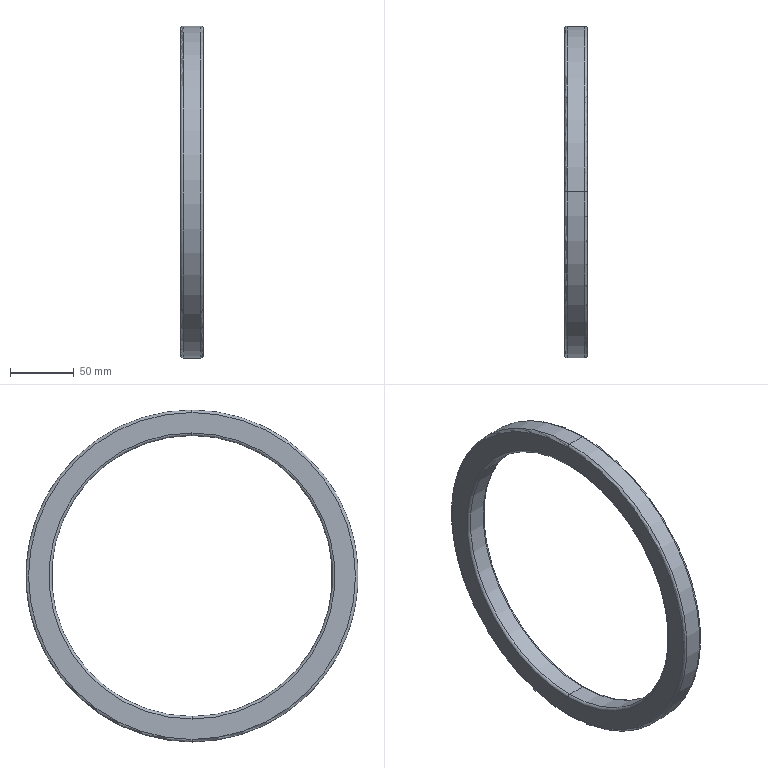Part | SolidWorks | features Revolution 1 | 1 solid | 35 faces | box 18 x 260 x 260 mm | volume 189235 mm3 | torus 20 | cylinder 10 | plane 5 | commonest cylinder face diameters 220 x2 230 x2 240 x2 250 x2 260 x2
STEP:
#1=CARTESIAN_POINT('',(5.,0.,123.));
#2=VERTEX_POINT('',#1);
#3=CARTESIAN_POINT('',(5.,0.,-123.));
#4=VERTEX_POINT('',#3);
#5=CARTESIAN_POINT('',(5.,0.,0.));
#6=DIRECTION('',(1.,0.,0.));
#7=DIRECTION('',(0.,0.,-1.));
#8=AXIS2_PLACEMENT_3D('',#5,#6,#7);
#9=CIRCLE('',#8,123.);
#10=EDGE_CURVE('',#2,#4,#9,.T.);
#11=ORIENTED_EDGE('',*,*,#10,.F.);
#12=CARTESIAN_POINT('',(7.,0.,125.));
#13=VERTEX_POINT('',#12);
#14=CARTESIAN_POINT('',(7.,0.,123.));
#15=DIRECTION('',(0.,1.,0.));
#16=DIRECTION('',(0.,0.,1.));
#17=AXIS2_PLACEMENT_3D('',#14,#15,#16);
#18=CIRCLE('',#17,2.);
#19=EDGE_CURVE('',#2,#13,#18,.T.);
#20=ORIENTED_EDGE('',*,*,#19,.T.);
#21=CARTESIAN_POINT('',(7.,0.,-125.));
#22=VERTEX_POINT('',#21);
#23=CARTESIAN_POINT('',(7.,0.,0.));
#24=DIRECTION('',(1.,0.,0.));
#25=DIRECTION('',(0.,0.,-1.));
#26=AXIS2_PLACEMENT_3D('',#23,#24,#25);
#27=CIRCLE('',#26,125.);
#28=EDGE_CURVE('',#13,#22,#27,.T.);
#29=ORIENTED_EDGE('',*,*,#28,.T.);
#30=CARTESIAN_POINT('',(7.,0.,-123.));
#31=DIRECTION('',(0.,-1.,0.));
#32=DIRECTION('',(0.,0.,-1.));
#33=AXIS2_PLACEMENT_3D('',#30,#31,#32);
#34=CIRCLE('',#33,2.);
#35=EDGE_CURVE('',#4,#22,#34,.T.);
#36=ORIENTED_EDGE('',*,*,#35,.F.);
#37=EDGE_LOOP('',(#11,#20,#29,#36));
#38=FACE_OUTER_BOUND('',#37,.T.);
#39=CARTESIAN_POINT('',(7.,0.,0.));
#40=DIRECTION('',(1.,0.,0.));
#41=DIRECTION('',(0.,0.,-1.));
#42=AXIS2_PLACEMENT_3D('',#39,#40,#41);
#43=TOROIDAL_SURFACE('',#42,123.,2.);
#44=ADVANCED_FACE('',(#38),#43,.F.);
#45=ORIENTED_EDGE('',*,*,#28,.F.);
#46=CARTESIAN_POINT('',(16.,0.,125.));
#47=VERTEX_POINT('',#46);
#48=CARTESIAN_POINT('',(119.308,0.,125.));
#49=DIRECTION('',(1.,0.,0.));
#50=VECTOR('',#49,1000.);
#51=LINE('',#48,#50);
#52=EDGE_CURVE('',#13,#47,#51,.T.);
#53=ORIENTED_EDGE('',*,*,#52,.T.);
#54=CARTESIAN_POINT('',(16.,0.,-125.));
#55=VERTEX_POINT('',#54);
#56=CARTESIAN_POINT('',(16.,0.,0.));
#57=DIRECTION('',(1.,0.,0.));
#58=DIRECTION('',(0.,0.,-1.));
#59=AXIS2_PLACEMENT_3D('',#56,#57,#58);
#60=CIRCLE('',#59,125.);
#61=EDGE_CURVE('',#47,#55,#60,.T.);
#62=ORIENTED_EDGE('',*,*,#61,.T.);
#63=CARTESIAN_POINT('',(119.308,0.,-125.));
#64=DIRECTION('',(1.,0.,0.));
#65=VECTOR('',#64,1000.);
#66=LINE('',#63,#65);
#67=EDGE_CURVE('',#22,#55,#66,.T.);
#68=ORIENTED_EDGE('',*,*,#67,.F.);
#69=EDGE_LOOP('',(#45,#53,#62,#68));
#70=FACE_OUTER_BOUND('',#69,.T.);
#71=CARTESIAN_POINT('',(119.308,0.,0.));
#72=DIRECTION('',(1.,0.,0.));
#73=DIRECTION('',(0.,0.,-1.));
#74=AXIS2_PLACEMENT_3D('',#71,#72,#73);
#75=CYLINDRICAL_SURFACE('',#74,125.);
#76=ADVANCED_FACE('',(#70),#75,.F.);
#77=CARTESIAN_POINT('',(18.,0.,-127.));
#78=VERTEX_POINT('',#77);
#79=CARTESIAN_POINT('',(18.,0.,127.));
#80=VERTEX_POINT('',#79);
#81=CARTESIAN_POINT('',(18.,0.,0.));
#82=DIRECTION('',(1.,0.,0.));
#83=DIRECTION('',(0.,0.,-1.));
#84=AXIS2_PLACEMENT_3D('',#81,#82,#83);
#85=CIRCLE('',#84,127.);
#86=EDGE_CURVE('',#78,#80,#85,.T.);
#87=ORIENTED_EDGE('',*,*,#86,.T.);
#88=CARTESIAN_POINT('',(16.,0.,127.));
#89=DIRECTION('',(0.,1.,0.));
#90=DIRECTION('',(0.,0.,1.));
#91=AXIS2_PLACEMENT_3D('',#88,#89,#90);
#92=CIRCLE('',#91,2.);
#93=EDGE_CURVE('',#80,#47,#92,.T.);
#94=ORIENTED_EDGE('',*,*,#93,.T.);
#95=CARTESIAN_POINT('',(16.,0.,0.));
#96=DIRECTION('',(1.,0.,0.));
#97=DIRECTION('',(0.,0.,-1.));
#98=AXIS2_PLACEMENT_3D('',#95,#96,#97);
#99=CIRCLE('',#98,125.);
#100=EDGE_CURVE('',#55,#47,#99,.T.);
#101=ORIENTED_EDGE('',*,*,#100,.F.);
#102=CARTESIAN_POINT('',(16.,0.,-127.));
#103=DIRECTION('',(0.,-1.,0.));
#104=DIRECTION('',(0.,0.,-1.));
#105=AXIS2_PLACEMENT_3D('',#102,#103,#104);
#106=CIRCLE('',#105,2.);
#107=EDGE_CURVE('',#78,#55,#106,.T.);
#108=ORIENTED_EDGE('',*,*,#107,.F.);
#109=EDGE_LOOP('',(#87,#94,#101,#108));
#110=FACE_OUTER_BOUND('',#109,.T.);
#111=CARTESIAN_POINT('',(16.,0.,0.));
#112=DIRECTION('',(1.,0.,0.));
#113=DIRECTION('',(0.,0.,-1.));
#114=AXIS2_PLACEMENT_3D('',#111,#112,#113);
#115=TOROIDAL_SURFACE('',#114,127.,2.);
#116=ADVANCED_FACE('',(#110),#115,.T.);
#117=CARTESIAN_POINT('',(16.,0.,-130.));
#118=VERTEX_POINT('',#117);
#119=CARTESIAN_POINT('',(16.,0.,130.));
#120=VERTEX_POINT('',#119);
#121=CARTESIAN_POINT('',(16.,0.,0.));
#122=DIRECTION('',(1.,0.,0.));
#123=DIRECTION('',(0.,0.,-1.));
#124=AXIS2_PLACEMENT_3D('',#121,#122,#123);
#125=CIRCLE('',#124,130.);
#126=EDGE_CURVE('',#118,#120,#125,.T.);
#127=ORIENTED_EDGE('',*,*,#126,.T.);
#128=CARTESIAN_POINT('',(18.,0.,128.));
#129=VERTEX_POINT('',#128);
#130=CARTESIAN_POINT('',(16.,0.,128.));
#131=DIRECTION('',(0.,1.,0.));
#132=DIRECTION('',(0.,0.,1.));
#133=AXIS2_PLACEMENT_3D('',#130,#131,#132);
#134=CIRCLE('',#133,2.);
#135=EDGE_CURVE('',#120,#129,#134,.T.);
#136=ORIENTED_EDGE('',*,*,#135,.T.);
#137=CARTESIAN_POINT('',(18.,0.,-128.));
#138=VERTEX_POINT('',#137);
#139=CARTESIAN_POINT('',(18.,0.,0.));
#140=DIRECTION('',(1.,0.,0.));
#141=DIRECTION('',(0.,0.,-1.));
#142=AXIS2_PLACEMENT_3D('',#139,#140,#141);
#143=CIRCLE('',#142,128.);
#144=EDGE_CURVE('',#138,#129,#143,.T.);
#145=ORIENTED_EDGE('',*,*,#144,.F.);
#146=CARTESIAN_POINT('',(16.,0.,-128.));
#147=DIRECTION('',(0.,-1.,0.));
#148=DIRECTION('',(0.,0.,-1.));
#149=AXIS2_PLACEMENT_3D('',#146,#147,#148);
#150=CIRCLE('',#149,2.);
#151=EDGE_CURVE('',#118,#138,#150,.T.);
#152=ORIENTED_EDGE('',*,*,#151,.F.);
#153=EDGE_LOOP('',(#127,#136,#145,#152));
#154=FACE_OUTER_BOUND('',#153,.T.);
#155=CARTESIAN_POINT('',(16.,0.,0.));
#156=DIRECTION('',(1.,0.,0.));
#157=DIRECTION('',(0.,0.,-1.));
#158=AXIS2_PLACEMENT_3D('',#155,#156,#157);
#159=TOROIDAL_SURFACE('',#158,128.,2.);
#160=ADVANCED_FACE('',(#154),#159,.T.);
#161=CARTESIAN_POINT('',(2.,0.,-130.));
#162=VERTEX_POINT('',#161);
#163=CARTESIAN_POINT('',(2.,0.,130.));
#164=VERTEX_POINT('',#163);
#165=CARTESIAN_POINT('',(2.,0.,0.));
#166=DIRECTION('',(1.,0.,0.));
#167=DIRECTION('',(0.,0.,-1.));
#168=AXIS2_PLACEMENT_3D('',#165,#166,#167);
#169=CIRCLE('',#168,130.);
#170=EDGE_CURVE('',#162,#164,#169,.T.);
#171=ORIENTED_EDGE('',*,*,#170,.T.);
#172=CARTESIAN_POINT('',(119.308,0.,130.));
#173=DIRECTION('',(1.,0.,0.));
#174=VECTOR('',#173,1000.);
#175=LINE('',#172,#174);
#176=EDGE_CURVE('',#164,#120,#175,.T.);
#177=ORIENTED_EDGE('',*,*,#176,.T.);
#178=ORIENTED_EDGE('',*,*,#126,.F.);
#179=CARTESIAN_POINT('',(119.308,0.,-130.));
#180=DIRECTION('',(1.,0.,0.));
#181=VECTOR('',#180,1000.);
#182=LINE('',#179,#181);
#183=EDGE_CURVE('',#162,#118,#182,.T.);
#184=ORIENTED_EDGE('',*,*,#183,.F.);
#185=EDGE_LOOP('',(#171,#177,#178,#184));
#186=FACE_OUTER_BOUND('',#185,.T.);
#187=CARTESIAN_POINT('',(119.308,0.,0.));
#188=DIRECTION('',(1.,0.,0.));
#189=DIRECTION('',(0.,0.,-1.));
#190=AXIS2_PLACEMENT_3D('',#187,#188,#189);
#191=CYLINDRICAL_SURFACE('',#190,130.);
#192=ADVANCED_FACE('',(#186),#191,.T.);
#193=CARTESIAN_POINT('',(0.,0.,-128.));
#194=VERTEX_POINT('',#193);
#195=CARTESIAN_POINT('',(0.,0.,128.));
#196=VERTEX_POINT('',#195);
#197=CARTESIAN_POINT('',(0.,0.,0.));
#198=DIRECTION('',(1.,0.,0.));
#199=DIRECTION('',(0.,0.,-1.));
#200=AXIS2_PLACEMENT_3D('',#197,#198,#199);
#201=CIRCLE('',#200,128.);
#202=EDGE_CURVE('',#194,#196,#201,.T.);
#203=ORIENTED_EDGE('',*,*,#202,.T.);
#204=CARTESIAN_POINT('',(2.,0.,128.));
#205=DIRECTION('',(0.,1.,0.));
#206=DIRECTION('',(0.,0.,1.));
#207=AXIS2_PLACEMENT_3D('',#204,#205,#206);
#208=CIRCLE('',#207,2.);
#209=EDGE_CURVE('',#196,#164,#208,.T.);
#210=ORIENTED_EDGE('',*,*,#209,.T.);
#211=ORIENTED_EDGE('',*,*,#170,.F.);
#212=CARTESIAN_POINT('',(2.,0.,-128.));
#213=DIRECTION('',(0.,-1.,0.));
#214=DIRECTION('',(0.,0.,-1.));
#215=AXIS2_PLACEMENT_3D('',#212,#213,#214);
#216=CIRCLE('',#215,2.);
#217=EDGE_CURVE('',#194,#162,#216,.T.);
#218=ORIENTED_EDGE('',*,*,#217,.F.);
#219=EDGE_LOOP('',(#203,#210,#211,#218));
#220=FACE_OUTER_BOUND('',#219,.T.);
#221=CARTESIAN_POINT('',(2.,0.,0.));
#222=DIRECTION('',(1.,0.,0.));
#223=DIRECTION('',(0.,0.,-1.));
#224=AXIS2_PLACEMENT_3D('',#221,#222,#223);
#225=TOROIDAL_SURFACE('',#224,128.,2.);
#226=ADVANCED_FACE('',(#220),#225,.T.);
#227=CARTESIAN_POINT('',(2.,0.,-110.));
#228=VERTEX_POINT('',#227);
#229=CARTESIAN_POINT('',(2.,0.,110.));
#230=VERTEX_POINT('',#229);
#231=CARTESIAN_POINT('',(2.,0.,0.));
#232=DIRECTION('',(1.,0.,0.));
#233=DIRECTION('',(0.,0.,-1.));
#234=AXIS2_PLACEMENT_3D('',#231,#232,#233);
#235=CIRCLE('',#234,110.);
#236=EDGE_CURVE('',#228,#230,#235,.T.);
#237=ORIENTED_EDGE('',*,*,#236,.T.);
#238=CARTESIAN_POINT('',(0.,0.,112.));
#239=VERTEX_POINT('',#238);
#240=CARTESIAN_POINT('',(2.,0.,112.));
#241=DIRECTION('',(0.,1.,0.));
#242=DIRECTION('',(0.,0.,1.));
#243=AXIS2_PLACEMENT_3D('',#240,#241,#242);
#244=CIRCLE('',#243,2.);
#245=EDGE_CURVE('',#230,#239,#244,.T.);
#246=ORIENTED_EDGE('',*,*,#245,.T.);
#247=CARTESIAN_POINT('',(0.,0.,-112.));
#248=VERTEX_POINT('',#247);
#249=CARTESIAN_POINT('',(0.,0.,0.));
#250=DIRECTION('',(1.,0.,0.));
#251=DIRECTION('',(0.,0.,-1.));
#252=AXIS2_PLACEMENT_3D('',#249,#250,#251);
#253=CIRCLE('',#252,112.);
#254=EDGE_CURVE('',#248,#239,#253,.T.);
#255=ORIENTED_EDGE('',*,*,#254,.F.);
#256=CARTESIAN_POINT('',(2.,0.,-112.));
#257=DIRECTION('',(0.,-1.,0.));
#258=DIRECTION('',(0.,0.,-1.));
#259=AXIS2_PLACEMENT_3D('',#256,#257,#258);
#260=CIRCLE('',#259,2.);
#261=EDGE_CURVE('',#228,#248,#260,.T.);
#262=ORIENTED_EDGE('',*,*,#261,.F.);
#263=EDGE_LOOP('',(#237,#246,#255,#262));
#264=FACE_OUTER_BOUND('',#263,.T.);
#265=CARTESIAN_POINT('',(2.,0.,0.));
#266=DIRECTION('',(1.,0.,0.));
#267=DIRECTION('',(0.,0.,-1.));
#268=AXIS2_PLACEMENT_3D('',#265,#266,#267);
#269=TOROIDAL_SURFACE('',#268,112.,2.);
#270=ADVANCED_FACE('',(#264),#269,.T.);
#271=CARTESIAN_POINT('',(2.,0.,0.));
#272=DIRECTION('',(1.,0.,0.));
#273=DIRECTION('',(0.,0.,-1.));
#274=AXIS2_PLACEMENT_3D('',#271,#272,#273);
#275=CIRCLE('',#274,110.);
#276=EDGE_CURVE('',#230,#228,#275,.T.);
#277=ORIENTED_EDGE('',*,*,#276,.F.);
#278=CARTESIAN_POINT('',(16.,0.,110.));
#279=VERTEX_POINT('',#278);
#280=CARTESIAN_POINT('',(119.308,0.,110.));
#281=DIRECTION('',(1.,0.,0.));
#282=VECTOR('',#281,1000.);
#283=LINE('',#280,#282);
#284=EDGE_CURVE('',#230,#279,#283,.T.);
#285=ORIENTED_EDGE('',*,*,#284,.T.);
#286=CARTESIAN_POINT('',(16.,0.,-110.));
#287=VERTEX_POINT('',#286);
#288=CARTESIAN_POINT('',(16.,0.,0.));
#289=DIRECTION('',(1.,0.,0.));
#290=DIRECTION('',(0.,0.,-1.));
#291=AXIS2_PLACEMENT_3D('',#288,#289,#290);
#292=CIRCLE('',#291,110.);
#293=EDGE_CURVE('',#279,#287,#292,.T.);
#294=ORIENTED_EDGE('',*,*,#293,.T.);
#295=CARTESIAN_POINT('',(119.308,0.,-110.));
#296=DIRECTION('',(1.,0.,0.));
#297=VECTOR('',#296,1000.);
#298=LINE('',#295,#297);
#299=EDGE_CURVE('',#228,#287,#298,.T.);
#300=ORIENTED_EDGE('',*,*,#299,.F.);
#301=EDGE_LOOP('',(#277,#285,#294,#300));
#302=FACE_OUTER_BOUND('',#301,.T.);
#303=CARTESIAN_POINT('',(119.308,0.,0.));
#304=DIRECTION('',(1.,0.,0.));
#305=DIRECTION('',(0.,0.,-1.));
#306=AXIS2_PLACEMENT_3D('',#303,#304,#305);
#307=CYLINDRICAL_SURFACE('',#306,110.);
#308=ADVANCED_FACE('',(#302),#307,.F.);
#309=CARTESIAN_POINT('',(18.,0.,-112.));
#310=VERTEX_POINT('',#309);
#311=CARTESIAN_POINT('',(18.,0.,112.));
#312=VERTEX_POINT('',#311);
#313=CARTESIAN_POINT('',(18.,0.,0.));
#314=DIRECTION('',(1.,0.,0.));
#315=DIRECTION('',(0.,0.,-1.));
#316=AXIS2_PLACEMENT_3D('',#313,#314,#315);
#317=CIRCLE('',#316,112.);
#318=EDGE_CURVE('',#310,#312,#317,.T.);
#319=ORIENTED_EDGE('',*,*,#318,.T.);
#320=CARTESIAN_POINT('',(16.,0.,112.));
#321=DIRECTION('',(0.,1.,0.));
#322=DIRECTION('',(0.,0.,1.));
#323=AXIS2_PLACEMENT_3D('',#320,#321,#322);
#324=CIRCLE('',#323,2.);
#325=EDGE_CURVE('',#312,#279,#324,.T.);
#326=ORIENTED_EDGE('',*,*,#325,.T.);
#327=CARTESIAN_POINT('',(16.,0.,0.));
#328=DIRECTION('',(1.,0.,0.));
#329=DIRECTION('',(0.,0.,-1.));
#330=AXIS2_PLACEMENT_3D('',#327,#328,#329);
#331=CIRCLE('',#330,110.);
#332=EDGE_CURVE('',#287,#279,#331,.T.);
#333=ORIENTED_EDGE('',*,*,#332,.F.);
#334=CARTESIAN_POINT('',(16.,0.,-112.));
#335=DIRECTION('',(0.,-1.,0.));
#336=DIRECTION('',(0.,0.,-1.));
#337=AXIS2_PLACEMENT_3D('',#334,#335,#336);
#338=CIRCLE('',#337,2.);
#339=EDGE_CURVE('',#310,#287,#338,.T.);
#340=ORIENTED_EDGE('',*,*,#339,.F.);
#341=EDGE_LOOP('',(#319,#326,#333,#340));
#342=FACE_OUTER_BOUND('',#341,.T.);
#343=CARTESIAN_POINT('',(16.,0.,0.));
#344=DIRECTION('',(1.,0.,0.));
#345=DIRECTION('',(0.,0.,-1.));
#346=AXIS2_PLACEMENT_3D('',#343,#344,#345);
#347=TOROIDAL_SURFACE('',#346,112.,2.);
#348=ADVANCED_FACE('',(#342),#347,.T.);
#349=CARTESIAN_POINT('',(16.,0.,-120.));
#350=VERTEX_POINT('',#349);
#351=CARTESIAN_POINT('',(16.,0.,120.));
#352=VERTEX_POINT('',#351);
#353=CARTESIAN_POINT('',(16.,0.,0.));
#354=DIRECTION('',(1.,0.,0.));
#355=DIRECTION('',(0.,0.,-1.));
#356=AXIS2_PLACEMENT_3D('',#353,#354,#355);
#357=CIRCLE('',#356,120.);
#358=EDGE_CURVE('',#350,#352,#357,.T.);
#359=ORIENTED_EDGE('',*,*,#358,.T.);
#360=CARTESIAN_POINT('',(18.,0.,118.));
#361=VERTEX_POINT('',#360);
#362=CARTESIAN_POINT('',(16.,0.,118.));
#363=DIRECTION('',(0.,1.,0.));
#364=DIRECTION('',(0.,0.,1.));
#365=AXIS2_PLACEMENT_3D('',#362,#363,#364);
#366=CIRCLE('',#365,2.);
#367=EDGE_CURVE('',#352,#361,#366,.T.);
#368=ORIENTED_EDGE('',*,*,#367,.T.);
#369=CARTESIAN_POINT('',(18.,0.,-118.));
#370=VERTEX_POINT('',#369);
#371=CARTESIAN_POINT('',(18.,0.,0.));
#372=DIRECTION('',(1.,0.,0.));
#373=DIRECTION('',(0.,0.,-1.));
#374=AXIS2_PLACEMENT_3D('',#371,#372,#373);
#375=CIRCLE('',#374,118.);
#376=EDGE_CURVE('',#370,#361,#375,.T.);
#377=ORIENTED_EDGE('',*,*,#376,.F.);
#378=CARTESIAN_POINT('',(16.,0.,-118.));
#379=DIRECTION('',(0.,-1.,0.));
#380=DIRECTION('',(0.,0.,-1.));
#381=AXIS2_PLACEMENT_3D('',#378,#379,#380);
#382=CIRCLE('',#381,2.);
#383=EDGE_CURVE('',#350,#370,#382,.T.);
#384=ORIENTED_EDGE('',*,*,#383,.F.);
#385=EDGE_LOOP('',(#359,#368,#377,#384));
#386=FACE_OUTER_BOUND('',#385,.T.);
#387=CARTESIAN_POINT('',(16.,0.,0.));
#388=DIRECTION('',(1.,0.,0.));
#389=DIRECTION('',(0.,0.,-1.));
#390=AXIS2_PLACEMENT_3D('',#387,#388,#389);
#391=TOROIDAL_SURFACE('',#390,118.,2.);
#392=ADVANCED_FACE('',(#386),#391,.T.);
#393=CARTESIAN_POINT('',(15.,0.,-120.));
#394=VERTEX_POINT('',#393);
#395=CARTESIAN_POINT('',(15.,0.,120.));
#396=VERTEX_POINT('',#395);
#397=CARTESIAN_POINT('',(15.,0.,0.));
#398=DIRECTION('',(1.,0.,0.));
#399=DIRECTION('',(0.,0.,-1.));
#400=AXIS2_PLACEMENT_3D('',#397,#398,#399);
#401=CIRCLE('',#400,120.);
#402=EDGE_CURVE('',#394,#396,#401,.T.);
#403=ORIENTED_EDGE('',*,*,#402,.T.);
#404=CARTESIAN_POINT('',(119.308,0.,120.));
#405=DIRECTION('',(1.,0.,0.));
#406=VECTOR('',#405,1000.);
#407=LINE('',#404,#406);
#408=EDGE_CURVE('',#396,#352,#407,.T.);
#409=ORIENTED_EDGE('',*,*,#408,.T.);
#410=ORIENTED_EDGE('',*,*,#358,.F.);
#411=CARTESIAN_POINT('',(119.308,0.,-120.));
#412=DIRECTION('',(1.,0.,0.));
#413=VECTOR('',#412,1000.);
#414=LINE('',#411,#413);
#415=EDGE_CURVE('',#394,#350,#414,.T.);
#416=ORIENTED_EDGE('',*,*,#415,.F.);
#417=EDGE_LOOP('',(#403,#409,#410,#416));
#418=FACE_OUTER_BOUND('',#417,.T.);
#419=CARTESIAN_POINT('',(119.308,0.,0.));
#420=DIRECTION('',(1.,0.,0.));
#421=DIRECTION('',(0.,0.,-1.));
#422=AXIS2_PLACEMENT_3D('',#419,#420,#421);
#423=CYLINDRICAL_SURFACE('',#422,120.);
#424=ADVANCED_FACE('',(#418),#423,.T.);
#425=CARTESIAN_POINT('',(13.,0.,-118.));
#426=VERTEX_POINT('',#425);
#427=CARTESIAN_POINT('',(13.,0.,118.));
#428=VERTEX_POINT('',#427);
#429=CARTESIAN_POINT('',(13.,0.,0.));
#430=DIRECTION('',(1.,0.,0.));
#431=DIRECTION('',(0.,0.,-1.));
#432=AXIS2_PLACEMENT_3D('',#429,#430,#431);
#433=CIRCLE('',#432,118.);
#434=EDGE_CURVE('',#426,#428,#433,.T.);
#435=ORIENTED_EDGE('',*,*,#434,.T.);
#436=CARTESIAN_POINT('',(15.,0.,118.));
#437=DIRECTION('',(0.,1.,0.));
#438=DIRECTION('',(0.,0.,1.));
#439=AXIS2_PLACEMENT_3D('',#436,#437,#438);
#440=CIRCLE('',#439,2.);
#441=EDGE_CURVE('',#428,#396,#440,.T.);
#442=ORIENTED_EDGE('',*,*,#441,.T.);
#443=ORIENTED_EDGE('',*,*,#402,.F.);
#444=CARTESIAN_POINT('',(15.,0.,-118.));
#445=DIRECTION('',(0.,-1.,0.));
#446=DIRECTION('',(0.,0.,-1.));
#447=AXIS2_PLACEMENT_3D('',#444,#445,#446);
#448=CIRCLE('',#447,2.);
#449=EDGE_CURVE('',#426,#394,#448,.T.);
#450=ORIENTED_EDGE('',*,*,#449,.F.);
#451=EDGE_LOOP('',(#435,#442,#443,#450));
#452=FACE_OUTER_BOUND('',#451,.T.);
#453=CARTESIAN_POINT('',(15.,0.,0.));
#454=DIRECTION('',(1.,0.,0.));
#455=DIRECTION('',(0.,0.,-1.));
#456=AXIS2_PLACEMENT_3D('',#453,#454,#455);
#457=TOROIDAL_SURFACE('',#456,118.,2.);
#458=ADVANCED_FACE('',(#452),#457,.T.);
#459=CARTESIAN_POINT('',(13.,0.,117.));
#460=VERTEX_POINT('',#459);
#461=CARTESIAN_POINT('',(13.,0.,-117.));
#462=VERTEX_POINT('',#461);
#463=CARTESIAN_POINT('',(13.,0.,0.));
#464=DIRECTION('',(1.,0.,0.));
#465=DIRECTION('',(0.,0.,-1.));
#466=AXIS2_PLACEMENT_3D('',#463,#464,#465);
#467=CIRCLE('',#466,117.);
#468=EDGE_CURVE('',#460,#462,#467,.T.);
#469=ORIENTED_EDGE('',*,*,#468,.F.);
#470=CARTESIAN_POINT('',(11.,0.,115.));
#471=VERTEX_POINT('',#470);
#472=CARTESIAN_POINT('',(11.,0.,117.));
#473=DIRECTION('',(0.,1.,0.));
#474=DIRECTION('',(0.,0.,1.));
#475=AXIS2_PLACEMENT_3D('',#472,#473,#474);
#476=CIRCLE('',#475,2.);
#477=EDGE_CURVE('',#460,#471,#476,.T.);
#478=ORIENTED_EDGE('',*,*,#477,.T.);
#479=CARTESIAN_POINT('',(11.,0.,-115.));
#480=VERTEX_POINT('',#479);
#481=CARTESIAN_POINT('',(11.,0.,0.));
#482=DIRECTION('',(1.,0.,0.));
#483=DIRECTION('',(0.,0.,-1.));
#484=AXIS2_PLACEMENT_3D('',#481,#482,#483);
#485=CIRCLE('',#484,115.);
#486=EDGE_CURVE('',#471,#480,#485,.T.);
#487=ORIENTED_EDGE('',*,*,#486,.T.);
#488=CARTESIAN_POINT('',(11.,0.,-117.));
#489=DIRECTION('',(0.,-1.,0.));
#490=DIRECTION('',(0.,0.,-1.));
#491=AXIS2_PLACEMENT_3D('',#488,#489,#490);
#492=CIRCLE('',#491,2.);
#493=EDGE_CURVE('',#462,#480,#492,.T.);
#494=ORIENTED_EDGE('',*,*,#493,.F.);
#495=EDGE_LOOP('',(#469,#478,#487,#494));
#496=FACE_OUTER_BOUND('',#495,.T.);
#497=CARTESIAN_POINT('',(11.,0.,0.));
#498=DIRECTION('',(1.,0.,0.));
#499=DIRECTION('',(0.,0.,-1.));
#500=AXIS2_PLACEMENT_3D('',#497,#498,#499);
#501=TOROIDAL_SURFACE('',#500,117.,2.);
#502=ADVANCED_FACE('',(#496),#501,.F.);
#503=CARTESIAN_POINT('',(7.,0.,-115.));
#504=VERTEX_POINT('',#503);
#505=CARTESIAN_POINT('',(7.,0.,115.));
#506=VERTEX_POINT('',#505);
#507=CARTESIAN_POINT('',(7.,0.,0.));
#508=DIRECTION('',(1.,0.,0.));
#509=DIRECTION('',(0.,0.,-1.));
#510=AXIS2_PLACEMENT_3D('',#507,#508,#509);
#511=CIRCLE('',#510,115.);
#512=EDGE_CURVE('',#504,#506,#511,.T.);
#513=ORIENTED_EDGE('',*,*,#512,.T.);
#514=CARTESIAN_POINT('',(119.308,0.,115.));
#515=DIRECTION('',(1.,0.,0.));
#516=VECTOR('',#515,1000.);
#517=LINE('',#514,#516);
#518=EDGE_CURVE('',#506,#471,#517,.T.);
#519=ORIENTED_EDGE('',*,*,#518,.T.);
#520=CARTESIAN_POINT('',(11.,0.,0.));
#521=DIRECTION('',(1.,0.,0.));
#522=DIRECTION('',(0.,0.,-1.));
#523=AXIS2_PLACEMENT_3D('',#520,#521,#522);
#524=CIRCLE('',#523,115.);
#525=EDGE_CURVE('',#480,#471,#524,.T.);
#526=ORIENTED_EDGE('',*,*,#525,.F.);
#527=CARTESIAN_POINT('',(119.308,0.,-115.));
#528=DIRECTION('',(1.,0.,0.));
#529=VECTOR('',#528,1000.);
#530=LINE('',#527,#529);
#531=EDGE_CURVE('',#504,#480,#530,.T.);
#532=ORIENTED_EDGE('',*,*,#531,.F.);
#533=EDGE_LOOP('',(#513,#519,#526,#532));
#534=FACE_OUTER_BOUND('',#533,.T.);
#535=CARTESIAN_POINT('',(119.308,0.,0.));
#536=DIRECTION('',(1.,0.,0.));
#537=DIRECTION('',(0.,0.,-1.));
#538=AXIS2_PLACEMENT_3D('',#535,#536,#537);
#539=CYLINDRICAL_SURFACE('',#538,115.);
#540=ADVANCED_FACE('',(#534),#539,.T.);
#541=CARTESIAN_POINT('',(7.,0.,0.));
#542=DIRECTION('',(1.,0.,0.));
#543=DIRECTION('',(0.,0.,-1.));
#544=AXIS2_PLACEMENT_3D('',#541,#542,#543);
#545=CIRCLE('',#544,115.);
#546=EDGE_CURVE('',#506,#504,#545,.T.);
#547=ORIENTED_EDGE('',*,*,#546,.F.);
#548=CARTESIAN_POINT('',(5.,0.,117.));
#549=VERTEX_POINT('',#548);
#550=CARTESIAN_POINT('',(7.,0.,117.));
#551=DIRECTION('',(0.,1.,0.));
#552=DIRECTION('',(0.,0.,1.));
#553=AXIS2_PLACEMENT_3D('',#550,#551,#552);
#554=CIRCLE('',#553,2.);
#555=EDGE_CURVE('',#506,#549,#554,.T.);
#556=ORIENTED_EDGE('',*,*,#555,.T.);
#557=CARTESIAN_POINT('',(5.,0.,-117.));
#558=VERTEX_POINT('',#557);
#559=CARTESIAN_POINT('',(5.,0.,0.));
#560=DIRECTION('',(1.,0.,0.));
#561=DIRECTION('',(0.,0.,-1.));
#562=AXIS2_PLACEMENT_3D('',#559,#560,#561);
#563=CIRCLE('',#562,117.);
#564=EDGE_CURVE('',#549,#558,#563,.T.);
#565=ORIENTED_EDGE('',*,*,#564,.T.);
#566=CARTESIAN_POINT('',(7.,0.,-117.));
#567=DIRECTION('',(0.,-1.,0.));
#568=DIRECTION('',(0.,0.,-1.));
#569=AXIS2_PLACEMENT_3D('',#566,#567,#568);
#570=CIRCLE('',#569,2.);
#571=EDGE_CURVE('',#504,#558,#570,.T.);
#572=ORIENTED_EDGE('',*,*,#571,.F.);
#573=EDGE_LOOP('',(#547,#556,#565,#572));
#574=FACE_OUTER_BOUND('',#573,.T.);
#575=CARTESIAN_POINT('',(7.,0.,0.));
#576=DIRECTION('',(1.,0.,0.));
#577=DIRECTION('',(0.,0.,-1.));
#578=AXIS2_PLACEMENT_3D('',#575,#576,#577);
#579=TOROIDAL_SURFACE('',#578,117.,2.);
#580=ADVANCED_FACE('',(#574),#579,.F.);
#581=ORIENTED_EDGE('',*,*,#555,.F.);
#582=ORIENTED_EDGE('',*,*,#512,.F.);
#583=ORIENTED_EDGE('',*,*,#571,.T.);
#584=CARTESIAN_POINT('',(5.,0.,0.));
#585=DIRECTION('',(1.,0.,0.));
#586=DIRECTION('',(0.,0.,-1.));
#587=AXIS2_PLACEMENT_3D('',#584,#585,#586);
#588=CIRCLE('',#587,117.);
#589=EDGE_CURVE('',#558,#549,#588,.T.);
#590=ORIENTED_EDGE('',*,*,#589,.T.);
#591=EDGE_LOOP('',(#581,#582,#583,#590));
#592=FACE_OUTER_BOUND('',#591,.T.);
#593=CARTESIAN_POINT('',(7.,0.,0.));
#594=DIRECTION('',(1.,0.,0.));
#595=DIRECTION('',(0.,0.,-1.));
#596=AXIS2_PLACEMENT_3D('',#593,#594,#595);
#597=TOROIDAL_SURFACE('',#596,117.,2.);
#598=ADVANCED_FACE('',(#592),#597,.F.);
#599=ORIENTED_EDGE('',*,*,#518,.F.);
#600=ORIENTED_EDGE('',*,*,#546,.T.);
#601=ORIENTED_EDGE('',*,*,#531,.T.);
#602=ORIENTED_EDGE('',*,*,#486,.F.);
#603=EDGE_LOOP('',(#599,#600,#601,#602));
#604=FACE_OUTER_BOUND('',#603,.T.);
#605=CARTESIAN_POINT('',(119.308,0.,0.));
#606=DIRECTION('',(1.,0.,0.));
#607=DIRECTION('',(0.,0.,-1.));
#608=AXIS2_PLACEMENT_3D('',#605,#606,#607);
#609=CYLINDRICAL_SURFACE('',#608,115.);
#610=ADVANCED_FACE('',(#604),#609,.T.);
#611=ORIENTED_EDGE('',*,*,#477,.F.);
#612=CARTESIAN_POINT('',(13.,0.,0.));
#613=DIRECTION('',(1.,0.,0.));
#614=DIRECTION('',(0.,0.,-1.));
#615=AXIS2_PLACEMENT_3D('',#612,#613,#614);
#616=CIRCLE('',#615,117.);
#617=EDGE_CURVE('',#462,#460,#616,.T.);
#618=ORIENTED_EDGE('',*,*,#617,.F.);
#619=ORIENTED_EDGE('',*,*,#493,.T.);
#620=ORIENTED_EDGE('',*,*,#525,.T.);
#621=EDGE_LOOP('',(#611,#618,#619,#620));
#622=FACE_OUTER_BOUND('',#621,.T.);
#623=CARTESIAN_POINT('',(11.,0.,0.));
#624=DIRECTION('',(1.,0.,0.));
#625=DIRECTION('',(0.,0.,-1.));
#626=AXIS2_PLACEMENT_3D('',#623,#624,#625);
#627=TOROIDAL_SURFACE('',#626,117.,2.);
#628=ADVANCED_FACE('',(#622),#627,.F.);
#629=ORIENTED_EDGE('',*,*,#617,.T.);
#630=ORIENTED_EDGE('',*,*,#468,.T.);
#631=EDGE_LOOP('',(#629,#630));
#632=FACE_BOUND('',#631,.T.);
#633=ORIENTED_EDGE('',*,*,#434,.F.);
#634=CARTESIAN_POINT('',(13.,0.,0.));
#635=DIRECTION('',(1.,0.,0.));
#636=DIRECTION('',(0.,0.,-1.));
#637=AXIS2_PLACEMENT_3D('',#634,#635,#636);
#638=CIRCLE('',#637,118.);
#639=EDGE_CURVE('',#428,#426,#638,.T.);
#640=ORIENTED_EDGE('',*,*,#639,.F.);
#641=EDGE_LOOP('',(#633,#640));
#642=FACE_OUTER_BOUND('',#641,.T.);
#643=CARTESIAN_POINT('',(13.,117.,0.));
#644=DIRECTION('',(-1.,0.,0.));
#645=DIRECTION('',(0.,0.,1.));
#646=AXIS2_PLACEMENT_3D('',#643,#644,#645);
#647=PLANE('',#646);
#648=ADVANCED_FACE('',(#632,#642),#647,.T.);
#649=ORIENTED_EDGE('',*,*,#441,.F.);
#650=ORIENTED_EDGE('',*,*,#639,.T.);
#651=ORIENTED_EDGE('',*,*,#449,.T.);
#652=CARTESIAN_POINT('',(15.,0.,0.));
#653=DIRECTION('',(1.,0.,0.));
#654=DIRECTION('',(0.,0.,-1.));
#655=AXIS2_PLACEMENT_3D('',#652,#653,#654);
#656=CIRCLE('',#655,120.);
#657=EDGE_CURVE('',#396,#394,#656,.T.);
#658=ORIENTED_EDGE('',*,*,#657,.F.);
#659=EDGE_LOOP('',(#649,#650,#651,#658));
#660=FACE_OUTER_BOUND('',#659,.T.);
#661=CARTESIAN_POINT('',(15.,0.,0.));
#662=DIRECTION('',(1.,0.,0.));
#663=DIRECTION('',(0.,0.,-1.));
#664=AXIS2_PLACEMENT_3D('',#661,#662,#663);
#665=TOROIDAL_SURFACE('',#664,118.,2.);
#666=ADVANCED_FACE('',(#660),#665,.T.);
#667=ORIENTED_EDGE('',*,*,#408,.F.);
#668=ORIENTED_EDGE('',*,*,#657,.T.);
#669=ORIENTED_EDGE('',*,*,#415,.T.);
#670=CARTESIAN_POINT('',(16.,0.,0.));
#671=DIRECTION('',(1.,0.,0.));
#672=DIRECTION('',(0.,0.,-1.));
#673=AXIS2_PLACEMENT_3D('',#670,#671,#672);
#674=CIRCLE('',#673,120.);
#675=EDGE_CURVE('',#352,#350,#674,.T.);
#676=ORIENTED_EDGE('',*,*,#675,.F.);
#677=EDGE_LOOP('',(#667,#668,#669,#676));
#678=FACE_OUTER_BOUND('',#677,.T.);
#679=CARTESIAN_POINT('',(119.308,0.,0.));
#680=DIRECTION('',(1.,0.,0.));
#681=DIRECTION('',(0.,0.,-1.));
#682=AXIS2_PLACEMENT_3D('',#679,#680,#681);
#683=CYLINDRICAL_SURFACE('',#682,120.);
#684=ADVANCED_FACE('',(#678),#683,.T.);
#685=ORIENTED_EDGE('',*,*,#367,.F.);
#686=ORIENTED_EDGE('',*,*,#675,.T.);
#687=ORIENTED_EDGE('',*,*,#383,.T.);
#688=CARTESIAN_POINT('',(18.,0.,0.));
#689=DIRECTION('',(1.,0.,0.));
#690=DIRECTION('',(0.,0.,-1.));
#691=AXIS2_PLACEMENT_3D('',#688,#689,#690);
#692=CIRCLE('',#691,118.);
#693=EDGE_CURVE('',#361,#370,#692,.T.);
#694=ORIENTED_EDGE('',*,*,#693,.F.);
#695=EDGE_LOOP('',(#685,#686,#687,#694));
#696=FACE_OUTER_BOUND('',#695,.T.);
#697=CARTESIAN_POINT('',(16.,0.,0.));
#698=DIRECTION('',(1.,0.,0.));
#699=DIRECTION('',(0.,0.,-1.));
#700=AXIS2_PLACEMENT_3D('',#697,#698,#699);
#701=TOROIDAL_SURFACE('',#700,118.,2.);
#702=ADVANCED_FACE('',(#696),#701,.T.);
#703=ORIENTED_EDGE('',*,*,#376,.T.);
#704=ORIENTED_EDGE('',*,*,#693,.T.);
#705=EDGE_LOOP('',(#703,#704));
#706=FACE_OUTER_BOUND('',#705,.T.);
#707=ORIENTED_EDGE('',*,*,#318,.F.);
#708=CARTESIAN_POINT('',(18.,0.,0.));
#709=DIRECTION('',(1.,0.,0.));
#710=DIRECTION('',(0.,0.,-1.));
#711=AXIS2_PLACEMENT_3D('',#708,#709,#710);
#712=CIRCLE('',#711,112.);
#713=EDGE_CURVE('',#312,#310,#712,.T.);
#714=ORIENTED_EDGE('',*,*,#713,.F.);
#715=EDGE_LOOP('',(#707,#714));
#716=FACE_BOUND('',#715,.T.);
#717=CARTESIAN_POINT('',(18.,112.,0.));
#718=DIRECTION('',(1.,0.,0.));
#719=DIRECTION('',(0.,0.,-1.));
#720=AXIS2_PLACEMENT_3D('',#717,#718,#719);
#721=PLANE('',#720);
#722=ADVANCED_FACE('',(#706,#716),#721,.T.);
#723=ORIENTED_EDGE('',*,*,#325,.F.);
#724=ORIENTED_EDGE('',*,*,#713,.T.);
#725=ORIENTED_EDGE('',*,*,#339,.T.);
#726=ORIENTED_EDGE('',*,*,#293,.F.);
#727=EDGE_LOOP('',(#723,#724,#725,#726));
#728=FACE_OUTER_BOUND('',#727,.T.);
#729=CARTESIAN_POINT('',(16.,0.,0.));
#730=DIRECTION('',(1.,0.,0.));
#731=DIRECTION('',(0.,0.,-1.));
#732=AXIS2_PLACEMENT_3D('',#729,#730,#731);
#733=TOROIDAL_SURFACE('',#732,112.,2.);
#734=ADVANCED_FACE('',(#728),#733,.T.);
#735=ORIENTED_EDGE('',*,*,#284,.F.);
#736=ORIENTED_EDGE('',*,*,#236,.F.);
#737=ORIENTED_EDGE('',*,*,#299,.T.);
#738=ORIENTED_EDGE('',*,*,#332,.T.);
#739=EDGE_LOOP('',(#735,#736,#737,#738));
#740=FACE_OUTER_BOUND('',#739,.T.);
#741=CARTESIAN_POINT('',(119.308,0.,0.));
#742=DIRECTION('',(1.,0.,0.));
#743=DIRECTION('',(0.,0.,-1.));
#744=AXIS2_PLACEMENT_3D('',#741,#742,#743);
#745=CYLINDRICAL_SURFACE('',#744,110.);
#746=ADVANCED_FACE('',(#740),#745,.F.);
#747=ORIENTED_EDGE('',*,*,#245,.F.);
#748=ORIENTED_EDGE('',*,*,#276,.T.);
#749=ORIENTED_EDGE('',*,*,#261,.T.);
#750=CARTESIAN_POINT('',(0.,0.,0.));
#751=DIRECTION('',(1.,0.,0.));
#752=DIRECTION('',(0.,0.,-1.));
#753=AXIS2_PLACEMENT_3D('',#750,#751,#752);
#754=CIRCLE('',#753,112.);
#755=EDGE_CURVE('',#239,#248,#754,.T.);
#756=ORIENTED_EDGE('',*,*,#755,.F.);
#757=EDGE_LOOP('',(#747,#748,#749,#756));
#758=FACE_OUTER_BOUND('',#757,.T.);
#759=CARTESIAN_POINT('',(2.,0.,0.));
#760=DIRECTION('',(1.,0.,0.));
#761=DIRECTION('',(0.,0.,-1.));
#762=AXIS2_PLACEMENT_3D('',#759,#760,#761);
#763=TOROIDAL_SURFACE('',#762,112.,2.);
#764=ADVANCED_FACE('',(#758),#763,.T.);
#765=ORIENTED_EDGE('',*,*,#254,.T.);
#766=ORIENTED_EDGE('',*,*,#755,.T.);
#767=EDGE_LOOP('',(#765,#766));
#768=FACE_BOUND('',#767,.T.);
#769=ORIENTED_EDGE('',*,*,#202,.F.);
#770=CARTESIAN_POINT('',(0.,0.,0.));
#771=DIRECTION('',(1.,0.,0.));
#772=DIRECTION('',(0.,0.,-1.));
#773=AXIS2_PLACEMENT_3D('',#770,#771,#772);
#774=CIRCLE('',#773,128.);
#775=EDGE_CURVE('',#196,#194,#774,.T.);
#776=ORIENTED_EDGE('',*,*,#775,.F.);
#777=EDGE_LOOP('',(#769,#776));
#778=FACE_OUTER_BOUND('',#777,.T.);
#779=CARTESIAN_POINT('',(0.,128.,0.));
#780=DIRECTION('',(-1.,0.,0.));
#781=DIRECTION('',(0.,0.,1.));
#782=AXIS2_PLACEMENT_3D('',#779,#780,#781);
#783=PLANE('',#782);
#784=ADVANCED_FACE('',(#768,#778),#783,.T.);
#785=ORIENTED_EDGE('',*,*,#209,.F.);
#786=ORIENTED_EDGE('',*,*,#775,.T.);
#787=ORIENTED_EDGE('',*,*,#217,.T.);
#788=CARTESIAN_POINT('',(2.,0.,0.));
#789=DIRECTION('',(1.,0.,0.));
#790=DIRECTION('',(0.,0.,-1.));
#791=AXIS2_PLACEMENT_3D('',#788,#789,#790);
#792=CIRCLE('',#791,130.);
#793=EDGE_CURVE('',#164,#162,#792,.T.);
#794=ORIENTED_EDGE('',*,*,#793,.F.);
#795=EDGE_LOOP('',(#785,#786,#787,#794));
#796=FACE_OUTER_BOUND('',#795,.T.);
#797=CARTESIAN_POINT('',(2.,0.,0.));
#798=DIRECTION('',(1.,0.,0.));
#799=DIRECTION('',(0.,0.,-1.));
#800=AXIS2_PLACEMENT_3D('',#797,#798,#799);
#801=TOROIDAL_SURFACE('',#800,128.,2.);
#802=ADVANCED_FACE('',(#796),#801,.T.);
#803=ORIENTED_EDGE('',*,*,#176,.F.);
#804=ORIENTED_EDGE('',*,*,#793,.T.);
#805=ORIENTED_EDGE('',*,*,#183,.T.);
#806=CARTESIAN_POINT('',(16.,0.,0.));
#807=DIRECTION('',(1.,0.,0.));
#808=DIRECTION('',(0.,0.,-1.));
#809=AXIS2_PLACEMENT_3D('',#806,#807,#808);
#810=CIRCLE('',#809,130.);
#811=EDGE_CURVE('',#120,#118,#810,.T.);
#812=ORIENTED_EDGE('',*,*,#811,.F.);
#813=EDGE_LOOP('',(#803,#804,#805,#812));
#814=FACE_OUTER_BOUND('',#813,.T.);
#815=CARTESIAN_POINT('',(119.308,0.,0.));
#816=DIRECTION('',(1.,0.,0.));
#817=DIRECTION('',(0.,0.,-1.));
#818=AXIS2_PLACEMENT_3D('',#815,#816,#817);
#819=CYLINDRICAL_SURFACE('',#818,130.);
#820=ADVANCED_FACE('',(#814),#819,.T.);
#821=ORIENTED_EDGE('',*,*,#135,.F.);
#822=ORIENTED_EDGE('',*,*,#811,.T.);
#823=ORIENTED_EDGE('',*,*,#151,.T.);
#824=CARTESIAN_POINT('',(18.,0.,0.));
#825=DIRECTION('',(1.,0.,0.));
#826=DIRECTION('',(0.,0.,-1.));
#827=AXIS2_PLACEMENT_3D('',#824,#825,#826);
#828=CIRCLE('',#827,128.);
#829=EDGE_CURVE('',#129,#138,#828,.T.);
#830=ORIENTED_EDGE('',*,*,#829,.F.);
#831=EDGE_LOOP('',(#821,#822,#823,#830));
#832=FACE_OUTER_BOUND('',#831,.T.);
#833=CARTESIAN_POINT('',(16.,0.,0.));
#834=DIRECTION('',(1.,0.,0.));
#835=DIRECTION('',(0.,0.,-1.));
#836=AXIS2_PLACEMENT_3D('',#833,#834,#835);
#837=TOROIDAL_SURFACE('',#836,128.,2.);
#838=ADVANCED_FACE('',(#832),#837,.T.);
#839=ORIENTED_EDGE('',*,*,#144,.T.);
#840=ORIENTED_EDGE('',*,*,#829,.T.);
#841=EDGE_LOOP('',(#839,#840));
#842=FACE_OUTER_BOUND('',#841,.T.);
#843=ORIENTED_EDGE('',*,*,#86,.F.);
#844=CARTESIAN_POINT('',(18.,0.,0.));
#845=DIRECTION('',(1.,0.,0.));
#846=DIRECTION('',(0.,0.,-1.));
#847=AXIS2_PLACEMENT_3D('',#844,#845,#846);
#848=CIRCLE('',#847,127.);
#849=EDGE_CURVE('',#80,#78,#848,.T.);
#850=ORIENTED_EDGE('',*,*,#849,.F.);
#851=EDGE_LOOP('',(#843,#850));
#852=FACE_BOUND('',#851,.T.);
#853=CARTESIAN_POINT('',(18.,128.,0.));
#854=DIRECTION('',(1.,0.,0.));
#855=DIRECTION('',(0.,0.,-1.));
#856=AXIS2_PLACEMENT_3D('',#853,#854,#855);
#857=PLANE('',#856);
#858=ADVANCED_FACE('',(#842,#852),#857,.T.);
#859=ORIENTED_EDGE('',*,*,#93,.F.);
#860=ORIENTED_EDGE('',*,*,#849,.T.);
#861=ORIENTED_EDGE('',*,*,#107,.T.);
#862=ORIENTED_EDGE('',*,*,#61,.F.);
#863=EDGE_LOOP('',(#859,#860,#861,#862));
#864=FACE_OUTER_BOUND('',#863,.T.);
#865=CARTESIAN_POINT('',(16.,0.,0.));
#866=DIRECTION('',(1.,0.,0.));
#867=DIRECTION('',(0.,0.,-1.));
#868=AXIS2_PLACEMENT_3D('',#865,#866,#867);
#869=TOROIDAL_SURFACE('',#868,127.,2.);
#870=ADVANCED_FACE('',(#864),#869,.T.);
#871=ORIENTED_EDGE('',*,*,#52,.F.);
#872=CARTESIAN_POINT('',(7.,0.,0.));
#873=DIRECTION('',(1.,0.,0.));
#874=DIRECTION('',(0.,0.,-1.));
#875=AXIS2_PLACEMENT_3D('',#872,#873,#874);
#876=CIRCLE('',#875,125.);
#877=EDGE_CURVE('',#22,#13,#876,.T.);
#878=ORIENTED_EDGE('',*,*,#877,.F.);
#879=ORIENTED_EDGE('',*,*,#67,.T.);
#880=ORIENTED_EDGE('',*,*,#100,.T.);
#881=EDGE_LOOP('',(#871,#878,#879,#880));
#882=FACE_OUTER_BOUND('',#881,.T.);
#883=CARTESIAN_POINT('',(119.308,0.,0.));
#884=DIRECTION('',(1.,0.,0.));
#885=DIRECTION('',(0.,0.,-1.));
#886=AXIS2_PLACEMENT_3D('',#883,#884,#885);
#887=CYLINDRICAL_SURFACE('',#886,125.);
#888=ADVANCED_FACE('',(#882),#887,.F.);
#889=ORIENTED_EDGE('',*,*,#19,.F.);
#890=CARTESIAN_POINT('',(5.,0.,0.));
#891=DIRECTION('',(1.,0.,0.));
#892=DIRECTION('',(0.,0.,-1.));
#893=AXIS2_PLACEMENT_3D('',#890,#891,#892);
#894=CIRCLE('',#893,123.);
#895=EDGE_CURVE('',#4,#2,#894,.T.);
#896=ORIENTED_EDGE('',*,*,#895,.F.);
#897=ORIENTED_EDGE('',*,*,#35,.T.);
#898=ORIENTED_EDGE('',*,*,#877,.T.);
#899=EDGE_LOOP('',(#889,#896,#897,#898));
#900=FACE_OUTER_BOUND('',#899,.T.);
#901=CARTESIAN_POINT('',(7.,0.,0.));
#902=DIRECTION('',(1.,0.,0.));
#903=DIRECTION('',(0.,0.,-1.));
#904=AXIS2_PLACEMENT_3D('',#901,#902,#903);
#905=TOROIDAL_SURFACE('',#904,123.,2.);
#906=ADVANCED_FACE('',(#900),#905,.F.);
#907=ORIENTED_EDGE('',*,*,#895,.T.);
#908=ORIENTED_EDGE('',*,*,#10,.T.);
#909=EDGE_LOOP('',(#907,#908));
#910=FACE_OUTER_BOUND('',#909,.T.);
#911=ORIENTED_EDGE('',*,*,#589,.F.);
#912=ORIENTED_EDGE('',*,*,#564,.F.);
#913=EDGE_LOOP('',(#911,#912));
#914=FACE_BOUND('',#913,.T.);
#915=CARTESIAN_POINT('',(5.,117.,0.));
#916=DIRECTION('',(1.,0.,0.));
#917=DIRECTION('',(0.,0.,-1.));
#918=AXIS2_PLACEMENT_3D('',#915,#916,#917);
#919=PLANE('',#918);
#920=ADVANCED_FACE('',(#910,#914),#919,.T.);
#921=CLOSED_SHELL('',(#44,#76,#116,#160,#192,#226,#270,#308,#348,#392,#424,#458,#502,#540,#580,#598,#610,#628,#648,#666,#684,#702,#722,#734,#746,#764,#784,#802,#820,#838,#858,#870,#888,#906,#920));
#922=MANIFOLD_SOLID_BREP('',#921);
#923=CARTESIAN_POINT('',(0.,0.,0.));
#924=DIRECTION('',(0.,0.,1.));
#925=DIRECTION('',(1.,0.,0.));
#926=AXIS2_PLACEMENT_3D('',#923,#924,#925);
#927=(LENGTH_UNIT()NAMED_UNIT(*)SI_UNIT(.MILLI.,.METRE.));
#928=UNCERTAINTY_MEASURE_WITH_UNIT(LENGTH_MEASURE(0.00001),#927,'','');
#929=(NAMED_UNIT(*)PLANE_ANGLE_UNIT()SI_UNIT($,.RADIAN.));
#930=(NAMED_UNIT(*)SI_UNIT($,.STERADIAN.)SOLID_ANGLE_UNIT());
#931=(GEOMETRIC_REPRESENTATION_CONTEXT(3)GLOBAL_UNCERTAINTY_ASSIGNED_CONTEXT((#928))GLOBAL_UNIT_ASSIGNED_CONTEXT((#927,#929,#930))REPRESENTATION_CONTEXT('',''));
#932=ADVANCED_BREP_SHAPE_REPRESENTATION('',(#922,#926),#931);